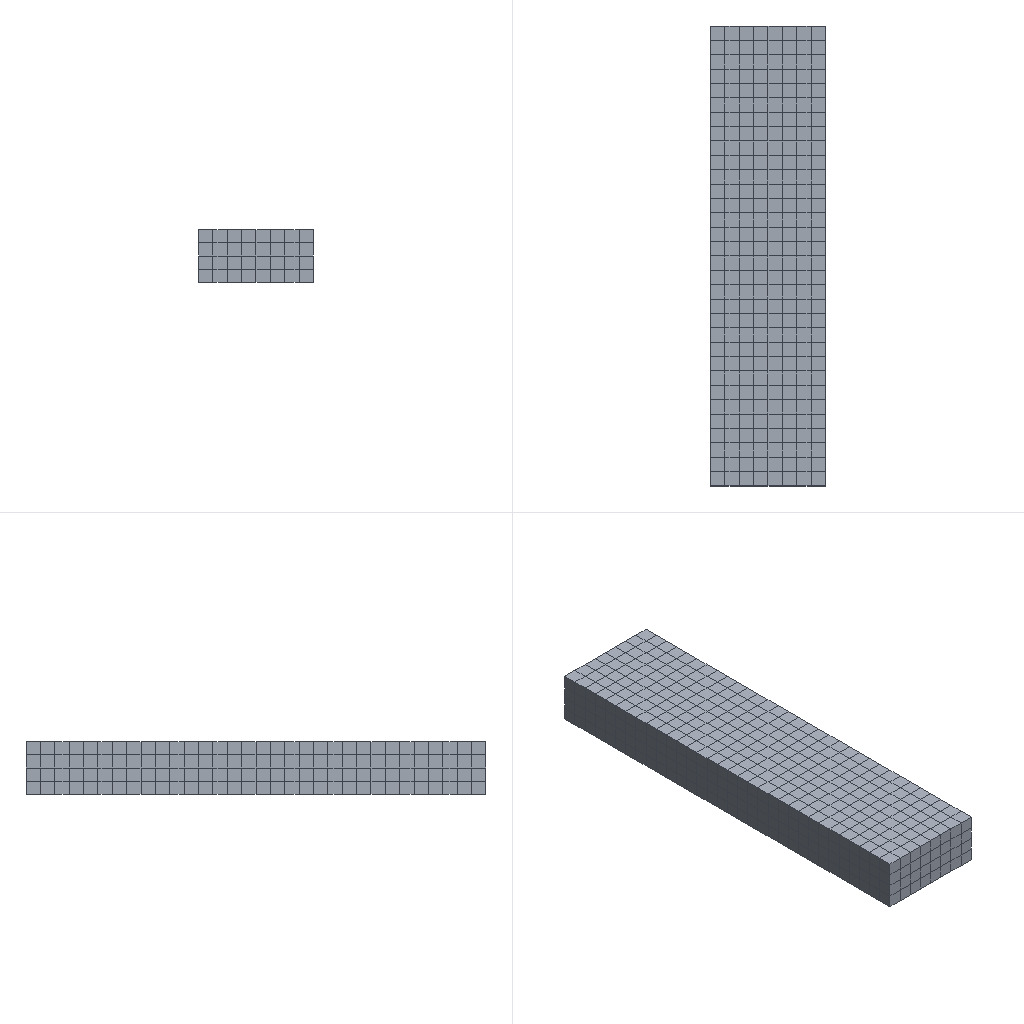Simulation study | abaqus
Set-up summary:
category,name,step,type,value,unit,region
solver,abaqus
solver,version,,,Abaqus/Standard 2020
units,not stated in the deck,,not stated
analysis,deck,,static,static
load_step,Step-1,Step-1,static
load_step,requested,,,1
mesh,nodes,,,1485
mesh,elements,,,1024
element_type,C3D8R,,solid,1024
load,load commands in deck,,count,1
bc,support commands in deck,,count,7
material,C45,,in results
material,C45-COPY,,in results
material,COH,,in results
material,H400,,in results
material,T63,,in results
check,setup vs results,,match,"per instance, exact: element labels, types and connectivity; labels of the nodes the elements use; coordinates of those nodes at SINGLE_PRECISION in 1 of 1 instance(s)"
Abaqus input file, long lists of numbers shortened:
*Heading
** Job name: Job-juxing Model name: Model-1-Copy-Copy
** Generated by: Abaqus/CAE 2020
*Preprint, echo=NO, model=NO, history=NO, contact=NO
**
** PARTS
**
*Part, name=con
*Node
      1,   543.297,        1650.,         250.
      2,   543.297,        -550.,         250.
** (1483 more lines like these left out)
*Element, type=C3D8R
   1,  158,  401,  835,  359,    1,   11,  173,   78
   2,  401,  402,  836,  835,   11,   12,  174,  173
** (1022 more lines like these left out)
*Nset, nset=Set-1, generate
    1,  1485,     1
*Elset, elset=Set-1, generate
    1,  1024,     1
** Section: con
*Solid Section, elset=Set-1, material=c45
,
*End Part
**
**
** ASSEMBLY
**
*Assembly, name=Assembly
**
*Instance, name=con-1, part=con
*End Instance
**
*Node
      1,   405.797,        -550.,         125.
*Nset, nset=Set-3, instance=con-1
   1,   4,   8,  10,  76,  77,  78, 142, 143, 144, 145, 146, 147, 148, 149, 150
 151, 152, 153, 154, 155, 156, 157, 158, 359, 360, 361, 362, 363, 364, 365, 366
** (1 more lines like these left out)
*Elset, elset=Set-3, instance=con-1, generate
   1,  993,   32
*Nset, nset=Set-8
 1,
*Nset, nset=m_Set-7
 1,
*Elset, elset=_s_Surf-1_S4, internal, instance=con-1, generate
   32,  1024,    32
*Surface, type=ELEMENT, name=s_Surf-1
_s_Surf-1_S4, S4
*Elset, elset=_s_Surf-2_S4, internal, instance=con-1, generate
   32,  1024,    32
*Surface, type=ELEMENT, name=s_Surf-2
_s_Surf-2_S4, S4
*Elset, elset=_s_Surf-3_S4, internal, instance=con-1, generate
   32,  1024,    32
*Surface, type=ELEMENT, name=s_Surf-3
_s_Surf-3_S4, S4
** Constraint: Constraint-2
*Coupling, constraint name=Constraint-2, ref node=m_Set-7, surface=s_Surf-3
*Kinematic
*End Assembly
*Amplitude, name=Amp-1
             0.,              0.,              1.,              1.
**
** MATERIALS
**
*Material, name=H400
*Density
 7.8e-09,
*Elastic
210000., 0.3
*Plastic
400.,0.
*Material, name=c45
*Density
 2.5e-09,
*Elastic
32500., 0.2
*Concrete Damaged Plasticity
30.,   0.1,  1.16, 0.667,  0.01
*Concrete Compression Hardening
 31.839,          0.
  35.238, 0.0001688
  37.656, 0.0002734
 39.058, 0.0004092
    39.5, 0.0005746
 38.815, 0.0007747
 37.101,  0.001006
  34.823,  0.001256
 32.332,  0.001511
 29.849,  0.001767
 27.497,  0.002018
 25.334,   0.002263
 23.376,  0.002503
 21.619,  0.002736
 20.051,  0.002963
 18.651,  0.003185
 17.402,  0.003403
 16.285,  0.003616
 15.284,  0.003826
 14.385,   0.004032
 13.573,  0.004236
 12.839,  0.004438
 12.173,  0.004637
 11.567,   0.004835
  11.013,  0.005031
*Concrete Tension Stiffening
  2.09,       0.
   2.4, 8.74e-06
  2.67, 1.23e-05
  2.86, 1.81e-05
  2.94, 2.75e-05
   2.8, 4.37e-05
  2.55, 6.31e-05
   2.3, 8.27e-05
  2.07, 0.000102
  1.86,  0.00012
  1.69, 0.000137
  1.55, 0.000153
  1.42, 0.000169
  1.31, 0.000184
  1.22, 0.000198
  1.14, 0.000213
  1.07, 0.000227
  1.01,  0.00024
 0.956, 0.000254
 0.908, 0.000267
 0.864,  0.00028
 0.825, 0.000293
 0.789, 0.000306
 0.757, 0.000319
 0.727, 0.000332
*Concrete Tension Damage, compression recovery=0.45
     0.,       0.
 0.0544, 8.74e-06
 0.0674, 1.23e-05
 0.0893, 1.81e-05
  0.124, 2.75e-05
  0.186, 4.37e-05
  0.255, 6.31e-05
  0.321, 8.27e-05
   0.38, 0.000102
  0.431,  0.00012
  0.475, 0.000137
  0.513, 0.000153
  0.546, 0.000169
  0.575, 0.000184
  0.601, 0.000198
  0.623, 0.000213
  0.643, 0.000227
  0.661,  0.00024
  0.678, 0.000254
  0.692, 0.000267
  0.706,  0.00028
  0.718, 0.000293
  0.729, 0.000306
  0.739, 0.000319
  0.749, 0.000332
  0.757, 0.000344
  0.765, 0.000357
  0.773, 0.000369
   0.78, 0.000382
  0.787, 0.000394
  0.793, 0.000407
  0.799, 0.000419
  0.804, 0.000431
  0.809, 0.000443
  0.814, 0.000456
  0.851, 0.000577
  0.875, 0.000697
  0.892, 0.000816
  0.905, 0.000935
  0.915,  0.00105
** (31 more lines like these left out)
*Material, name=c45-Copy
*Density
 2.5e-09,
*Elastic
32500., 0.2
*Concrete Damaged Plasticity
30.,   0.1,  1.16, 0.667,  0.01
*Concrete Compression Hardening
 31.839,          0.
  35.238, 0.0001688
  37.656, 0.0002734
 39.058, 0.0004092
    39.5, 0.0005746
 38.815, 0.0007747
 37.101,  0.001006
  34.823,  0.001256
 32.332,  0.001511
 29.849,  0.001767
 27.497,  0.002018
 25.334,   0.002263
 23.376,  0.002503
 21.619,  0.002736
 20.051,  0.002963
 18.651,  0.003185
 17.402,  0.003403
 16.285,  0.003616
 15.284,  0.003826
 14.385,   0.004032
 13.573,  0.004236
 12.839,  0.004438
 12.173,  0.004637
 11.567,   0.004835
  11.013,  0.005031
*Concrete Tension Stiffening
  2.09,       0.
   2.4, 8.74e-06
  2.67, 1.23e-05
  2.86, 1.81e-05
  2.94, 2.75e-05
   2.8, 4.37e-05
  2.55, 6.31e-05
   2.3, 8.27e-05
  2.07, 0.000102
  1.86,  0.00012
  1.69, 0.000137
  1.55, 0.000153
  1.42, 0.000169
  1.31, 0.000184
  1.22, 0.000198
  1.14, 0.000213
  1.07, 0.000227
  1.01,  0.00024
 0.956, 0.000254
 0.908, 0.000267
 0.864,  0.00028
 0.825, 0.000293
 0.789, 0.000306
 0.757, 0.000319
 0.727, 0.000332
*Concrete Compression Damage
        0.,          0.
 0.06977, 0.0001688
  0.1005, 0.0002734
  0.1363, 0.0004092
  0.176, 0.0005746
  0.2212, 0.0007747
  0.271,  0.001006
  0.3214,  0.001256
  0.3699,  0.001511
  0.4151,  0.001767
  0.4565,  0.002018
  0.4939,   0.002263
  0.5275,  0.002503
   0.5577,  0.002736
  0.5849,  0.002963
   0.6093,  0.003185
  0.6313,  0.003403
  0.6511,  0.003616
  0.6691,  0.003826
  0.6855,   0.004032
  0.7004,  0.004236
  0.7141,  0.004438
  0.7266,  0.004637
  0.7382,   0.004835
  0.7488,  0.005031
  0.7586,  0.005226
  0.7678,  0.005419
  0.7763,  0.005611
  0.7842,  0.005802
  0.7915,  0.005993
  0.7984,  0.006182
  0.8049,  0.006371
  0.811,  0.006559
  0.8167,  0.006747
  0.8221,  0.006933
  0.8627,  0.008781
  0.8884,   0.01061
  0.906,   0.01242
  0.9188,   0.01423
  0.9286,   0.01603
** (21 more lines like these left out)
*Concrete Tension Damage, compression recovery=0.45
     0.,       0.
 0.0544, 8.74e-06
 0.0674, 1.23e-05
 0.0893, 1.81e-05
  0.124, 2.75e-05
  0.186, 4.37e-05
  0.255, 6.31e-05
  0.321, 8.27e-05
   0.38, 0.000102
  0.431,  0.00012
  0.475, 0.000137
  0.513, 0.000153
  0.546, 0.000169
  0.575, 0.000184
  0.601, 0.000198
  0.623, 0.000213
  0.643, 0.000227
  0.661,  0.00024
  0.678, 0.000254
  0.692, 0.000267
  0.706,  0.00028
  0.718, 0.000293
  0.729, 0.000306
  0.739, 0.000319
  0.749, 0.000332
  0.757, 0.000344
  0.765, 0.000357
  0.773, 0.000369
   0.78, 0.000382
  0.787, 0.000394
  0.793, 0.000407
  0.799, 0.000419
  0.804, 0.000431
  0.809, 0.000443
  0.814, 0.000456
  0.851, 0.000577
  0.875, 0.000697
  0.892, 0.000816
  0.905, 0.000935
  0.915,  0.00105
** (31 more lines like these left out)
*Material, name=coh
*Damage Initiation, criterion=MAXS
10.,10.,10.
*Damage Evolution, type=DISPLACEMENT
 1e-05,
*Damage Stabilization
0.001
*Density
 2.5e-09,
*Elastic, type=TRACTION
20000.,20000.,20000.
*Material, name=t63
*Density
 7.8e-09,
*Elastic
210000., 0.3
*Plastic
630.,0.
** ----------------------------------------------------------------
**
** STEP: Step-1
**
*Step, name=Step-1, nlgeom=YES, inc=5000
*Static, stabilize=0.0002, allsdtol=0.05, continue=NO
0.01, 1., 1e-05, 1.
**
** BOUNDARY CONDITIONS
**
** Name: BC-1 Type: 对称/反对称/完全固定
*Boundary
Set-3, ENCASTRE
** Name: [REDACTED] : Displacement/rotation angle
*Boundary, amplitude=Amp-1
Set-8, 1, 1, 30.
Set-8, 2, 2
Set-8, 3, 3
Set-8, 4, 4
Set-8, 5, 5
Set-8, 6, 6
**
** OUTPUT REQUESTS
**
*Restart, write, number interval=1, time marks=NO
**
** FIELD OUTPUT: F-Output-1
**
*Output, field
*Node Output
CF, RF, RM, RT, U, V
*Element Output, directions=YES
DAMAGEC, DAMAGET, E, EVOL, LE, MISES, MISESMAX, MISESONLY, PE, PEEQ, PEEQMAX, PEEQT, PEMAG, S, SDEG, SF
SSAVG, STATUS, STH, SVOL, VEEQ, pfopen
*Contact Output
CDISP, CSTRESS
**
** HISTORY OUTPUT: H-Output-1
**
*Output, history
*Node Output, nset=Set-8
RF2, U2
*End Step
Results summary:
result,step,,completed,increments=92 time=1.0/1.0
result,analysis,,,static
result,last_loadstep,,,1
result,primary field,,,U
result,reaction total,,FX,2734.264,model units
result,reaction total,,FY,1066.782,model units
result,reaction total,,FZ,-0.0,model units